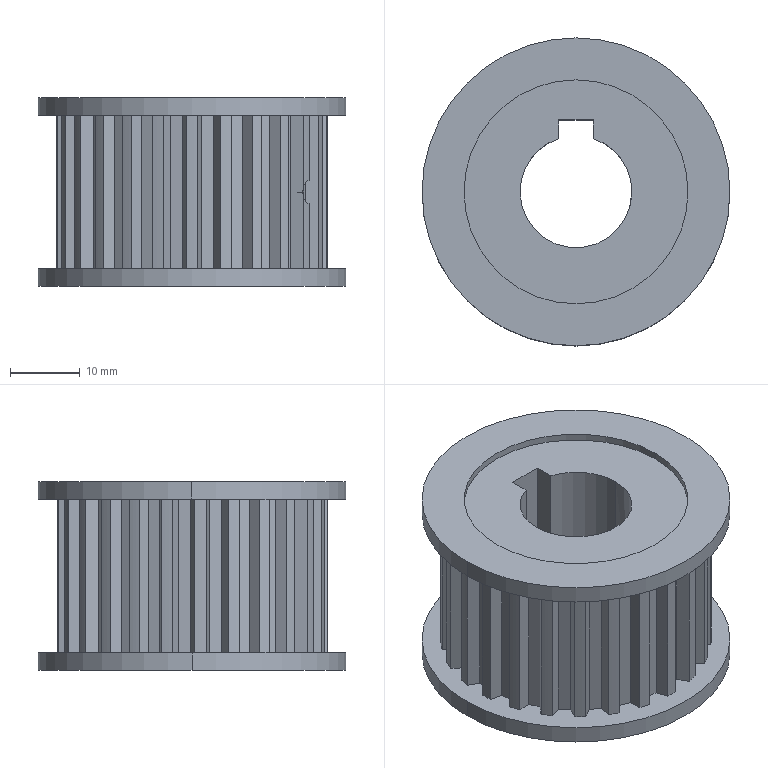Part | SolidWorks | features ICE 4, CirPattern 2, Fillet 2, MirrorPattern 2, Extrusion 1, HoleWzd 1 | 1 solid | 135 faces | box 44 x 44 x 27 mm | volume 23897 mm3 | plane 88 | cylinder 47 | commonest cylinder face diameters 38.65 x26 0.5 x4 3.3 x4 32 x4 44 x4 16 x3